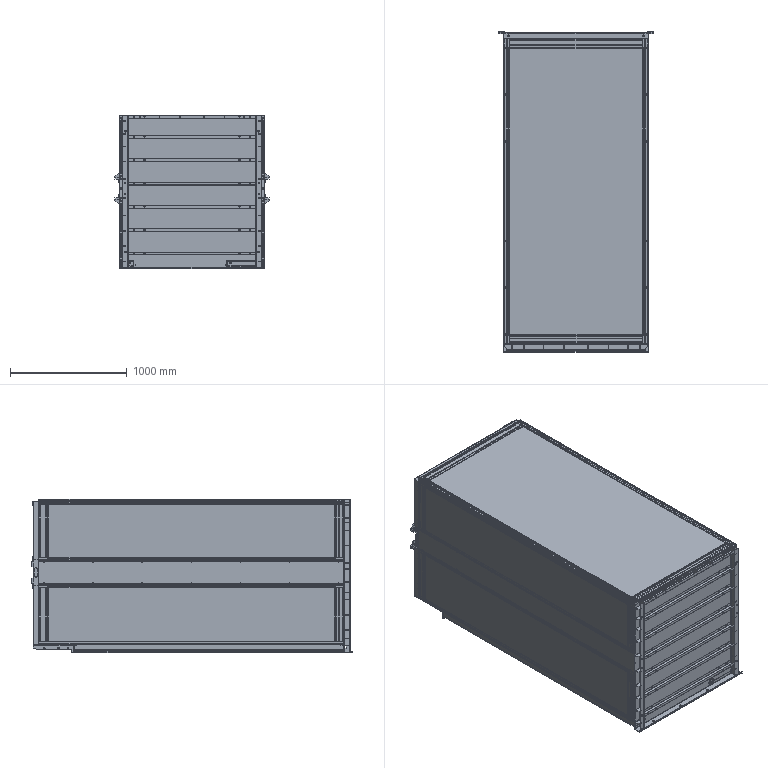Part | 147 solids | 6310 faces | volume 132240189 mm3 | plane 3860 | cylinder 2384 | cone 66 | commonest cylinder face diameters 0.4 x295 0.6 x232 13 x204 11 x195 10 x190 9 x152